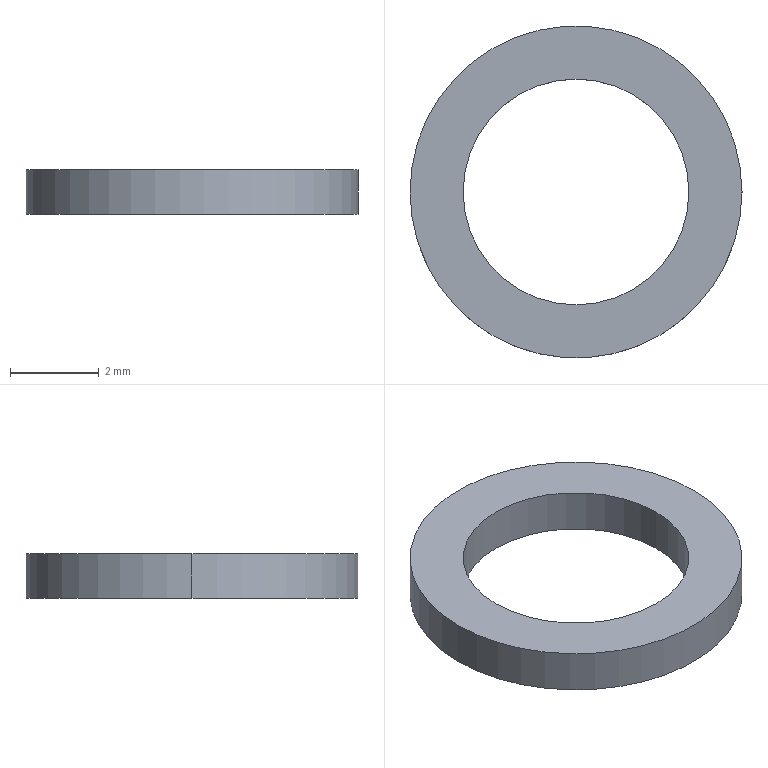Part | STEP file | PN_0010 Default | 1 solid | 6 faces | box 7.5 x 7.5 x 1 mm | volume 23.75 mm3 | cylinder 4 | plane 2 | commonest cylinder face diameters 5.1 x2 7.5 x2
STEP:
#1=CARTESIAN_POINT('',(-2.55,0.,1.));
#2=VERTEX_POINT('',#1);
#3=CARTESIAN_POINT('',(2.55,0.,1.));
#4=VERTEX_POINT('',#3);
#5=CARTESIAN_POINT('',(0.,0.,1.));
#6=DIRECTION('',(0.,0.,1.));
#7=DIRECTION('',(1.,0.,0.));
#8=AXIS2_PLACEMENT_3D('',#5,#6,#7);
#9=CIRCLE('',#8,2.55);
#10=EDGE_CURVE('',#2,#4,#9,.T.);
#11=ORIENTED_EDGE('',*,*,#10,.T.);
#12=CARTESIAN_POINT('',(2.55,0.,0.));
#13=VERTEX_POINT('',#12);
#14=CARTESIAN_POINT('',(2.55,0.,1.));
#15=DIRECTION('',(0.,0.,-1.));
#16=VECTOR('',#15,1000.);
#17=LINE('',#14,#16);
#18=EDGE_CURVE('',#4,#13,#17,.T.);
#19=ORIENTED_EDGE('',*,*,#18,.T.);
#20=CARTESIAN_POINT('',(-2.55,0.,0.));
#21=VERTEX_POINT('',#20);
#22=CARTESIAN_POINT('',(0.,0.,0.));
#23=DIRECTION('',(0.,0.,1.));
#24=DIRECTION('',(1.,0.,0.));
#25=AXIS2_PLACEMENT_3D('',#22,#23,#24);
#26=CIRCLE('',#25,2.55);
#27=EDGE_CURVE('',#21,#13,#26,.T.);
#28=ORIENTED_EDGE('',*,*,#27,.F.);
#29=CARTESIAN_POINT('',(-2.55,0.,1.));
#30=DIRECTION('',(0.,0.,-1.));
#31=VECTOR('',#30,1000.);
#32=LINE('',#29,#31);
#33=EDGE_CURVE('',#2,#21,#32,.T.);
#34=ORIENTED_EDGE('',*,*,#33,.F.);
#35=EDGE_LOOP('',(#11,#19,#28,#34));
#36=FACE_OUTER_BOUND('',#35,.T.);
#37=CARTESIAN_POINT('',(0.,0.,1.));
#38=DIRECTION('',(0.,0.,-1.));
#39=DIRECTION('',(-1.,0.,0.));
#40=AXIS2_PLACEMENT_3D('',#37,#38,#39);
#41=CYLINDRICAL_SURFACE('',#40,2.55);
#42=ADVANCED_FACE('',(#36),#41,.F.);
#43=CARTESIAN_POINT('',(3.75,0.,1.));
#44=VERTEX_POINT('',#43);
#45=CARTESIAN_POINT('',(-3.75,0.,1.));
#46=VERTEX_POINT('',#45);
#47=CARTESIAN_POINT('',(0.,0.,1.));
#48=DIRECTION('',(0.,0.,1.));
#49=DIRECTION('',(1.,0.,0.));
#50=AXIS2_PLACEMENT_3D('',#47,#48,#49);
#51=CIRCLE('',#50,3.75);
#52=EDGE_CURVE('',#44,#46,#51,.T.);
#53=ORIENTED_EDGE('',*,*,#52,.F.);
#54=CARTESIAN_POINT('',(3.75,0.,0.));
#55=VERTEX_POINT('',#54);
#56=CARTESIAN_POINT('',(3.75,0.,1.));
#57=DIRECTION('',(0.,0.,-1.));
#58=VECTOR('',#57,1000.);
#59=LINE('',#56,#58);
#60=EDGE_CURVE('',#44,#55,#59,.T.);
#61=ORIENTED_EDGE('',*,*,#60,.T.);
#62=CARTESIAN_POINT('',(-3.75,0.,0.));
#63=VERTEX_POINT('',#62);
#64=CARTESIAN_POINT('',(0.,0.,0.));
#65=DIRECTION('',(0.,0.,1.));
#66=DIRECTION('',(1.,0.,0.));
#67=AXIS2_PLACEMENT_3D('',#64,#65,#66);
#68=CIRCLE('',#67,3.75);
#69=EDGE_CURVE('',#55,#63,#68,.T.);
#70=ORIENTED_EDGE('',*,*,#69,.T.);
#71=CARTESIAN_POINT('',(-3.75,0.,1.));
#72=DIRECTION('',(0.,0.,-1.));
#73=VECTOR('',#72,1000.);
#74=LINE('',#71,#73);
#75=EDGE_CURVE('',#46,#63,#74,.T.);
#76=ORIENTED_EDGE('',*,*,#75,.F.);
#77=EDGE_LOOP('',(#53,#61,#70,#76));
#78=FACE_OUTER_BOUND('',#77,.T.);
#79=CARTESIAN_POINT('',(0.,0.,1.));
#80=DIRECTION('',(0.,0.,-1.));
#81=DIRECTION('',(-1.,0.,0.));
#82=AXIS2_PLACEMENT_3D('',#79,#80,#81);
#83=CYLINDRICAL_SURFACE('',#82,3.75);
#84=ADVANCED_FACE('',(#78),#83,.T.);
#85=CARTESIAN_POINT('',(0.,0.,1.));
#86=DIRECTION('',(0.,0.,1.));
#87=DIRECTION('',(1.,0.,0.));
#88=AXIS2_PLACEMENT_3D('',#85,#86,#87);
#89=CIRCLE('',#88,3.75);
#90=EDGE_CURVE('',#46,#44,#89,.T.);
#91=ORIENTED_EDGE('',*,*,#90,.T.);
#92=ORIENTED_EDGE('',*,*,#52,.T.);
#93=EDGE_LOOP('',(#91,#92));
#94=FACE_OUTER_BOUND('',#93,.T.);
#95=ORIENTED_EDGE('',*,*,#10,.F.);
#96=CARTESIAN_POINT('',(0.,0.,1.));
#97=DIRECTION('',(0.,0.,1.));
#98=DIRECTION('',(1.,0.,0.));
#99=AXIS2_PLACEMENT_3D('',#96,#97,#98);
#100=CIRCLE('',#99,2.55);
#101=EDGE_CURVE('',#4,#2,#100,.T.);
#102=ORIENTED_EDGE('',*,*,#101,.F.);
#103=EDGE_LOOP('',(#95,#102));
#104=FACE_BOUND('',#103,.T.);
#105=CARTESIAN_POINT('',(0.,0.,1.));
#106=DIRECTION('',(0.,0.,1.));
#107=DIRECTION('',(1.,0.,0.));
#108=AXIS2_PLACEMENT_3D('',#105,#106,#107);
#109=PLANE('',#108);
#110=ADVANCED_FACE('',(#94,#104),#109,.T.);
#111=CARTESIAN_POINT('',(0.,0.,0.));
#112=DIRECTION('',(0.,0.,1.));
#113=DIRECTION('',(1.,0.,0.));
#114=AXIS2_PLACEMENT_3D('',#111,#112,#113);
#115=CIRCLE('',#114,3.75);
#116=EDGE_CURVE('',#63,#55,#115,.T.);
#117=ORIENTED_EDGE('',*,*,#116,.F.);
#118=ORIENTED_EDGE('',*,*,#69,.F.);
#119=EDGE_LOOP('',(#117,#118));
#120=FACE_OUTER_BOUND('',#119,.T.);
#121=ORIENTED_EDGE('',*,*,#27,.T.);
#122=CARTESIAN_POINT('',(0.,0.,0.));
#123=DIRECTION('',(0.,0.,1.));
#124=DIRECTION('',(1.,0.,0.));
#125=AXIS2_PLACEMENT_3D('',#122,#123,#124);
#126=CIRCLE('',#125,2.55);
#127=EDGE_CURVE('',#13,#21,#126,.T.);
#128=ORIENTED_EDGE('',*,*,#127,.T.);
#129=EDGE_LOOP('',(#121,#128));
#130=FACE_BOUND('',#129,.T.);
#131=CARTESIAN_POINT('',(0.,0.,0.));
#132=DIRECTION('',(0.,0.,1.));
#133=DIRECTION('',(1.,0.,0.));
#134=AXIS2_PLACEMENT_3D('',#131,#132,#133);
#135=PLANE('',#134);
#136=ADVANCED_FACE('',(#120,#130),#135,.F.);
#137=ORIENTED_EDGE('',*,*,#60,.F.);
#138=ORIENTED_EDGE('',*,*,#90,.F.);
#139=ORIENTED_EDGE('',*,*,#75,.T.);
#140=ORIENTED_EDGE('',*,*,#116,.T.);
#141=EDGE_LOOP('',(#137,#138,#139,#140));
#142=FACE_OUTER_BOUND('',#141,.T.);
#143=CARTESIAN_POINT('',(0.,0.,1.));
#144=DIRECTION('',(0.,0.,-1.));
#145=DIRECTION('',(-1.,0.,0.));
#146=AXIS2_PLACEMENT_3D('',#143,#144,#145);
#147=CYLINDRICAL_SURFACE('',#146,3.75);
#148=ADVANCED_FACE('',(#142),#147,.T.);
#149=ORIENTED_EDGE('',*,*,#18,.F.);
#150=ORIENTED_EDGE('',*,*,#101,.T.);
#151=ORIENTED_EDGE('',*,*,#33,.T.);
#152=ORIENTED_EDGE('',*,*,#127,.F.);
#153=EDGE_LOOP('',(#149,#150,#151,#152));
#154=FACE_OUTER_BOUND('',#153,.T.);
#155=CARTESIAN_POINT('',(0.,0.,1.));
#156=DIRECTION('',(0.,0.,-1.));
#157=DIRECTION('',(-1.,0.,0.));
#158=AXIS2_PLACEMENT_3D('',#155,#156,#157);
#159=CYLINDRICAL_SURFACE('',#158,2.55);
#160=ADVANCED_FACE('',(#154),#159,.F.);
#161=CLOSED_SHELL('',(#42,#84,#110,#136,#148,#160));
#162=MANIFOLD_SOLID_BREP('',#161);
#163=CARTESIAN_POINT('',(0.,0.,0.));
#164=DIRECTION('',(0.,0.,1.));
#165=DIRECTION('',(1.,0.,0.));
#166=AXIS2_PLACEMENT_3D('',#163,#164,#165);
#167=(LENGTH_UNIT()NAMED_UNIT(*)SI_UNIT(.MILLI.,.METRE.));
#168=UNCERTAINTY_MEASURE_WITH_UNIT(LENGTH_MEASURE(0.00001),#167,'','');
#169=(NAMED_UNIT(*)PLANE_ANGLE_UNIT()SI_UNIT($,.RADIAN.));
#170=(NAMED_UNIT(*)SI_UNIT($,.STERADIAN.)SOLID_ANGLE_UNIT());
#171=(GEOMETRIC_REPRESENTATION_CONTEXT(3)GLOBAL_UNCERTAINTY_ASSIGNED_CONTEXT((#168))GLOBAL_UNIT_ASSIGNED_CONTEXT((#167,#169,#170))REPRESENTATION_CONTEXT('',''));
#172=ADVANCED_BREP_SHAPE_REPRESENTATION('',(#162,#166),#171);